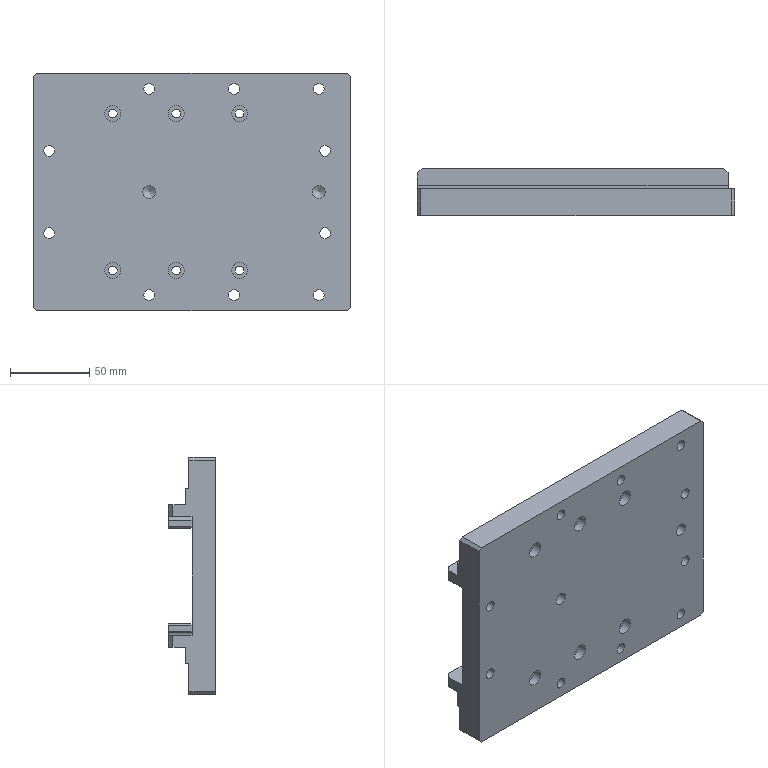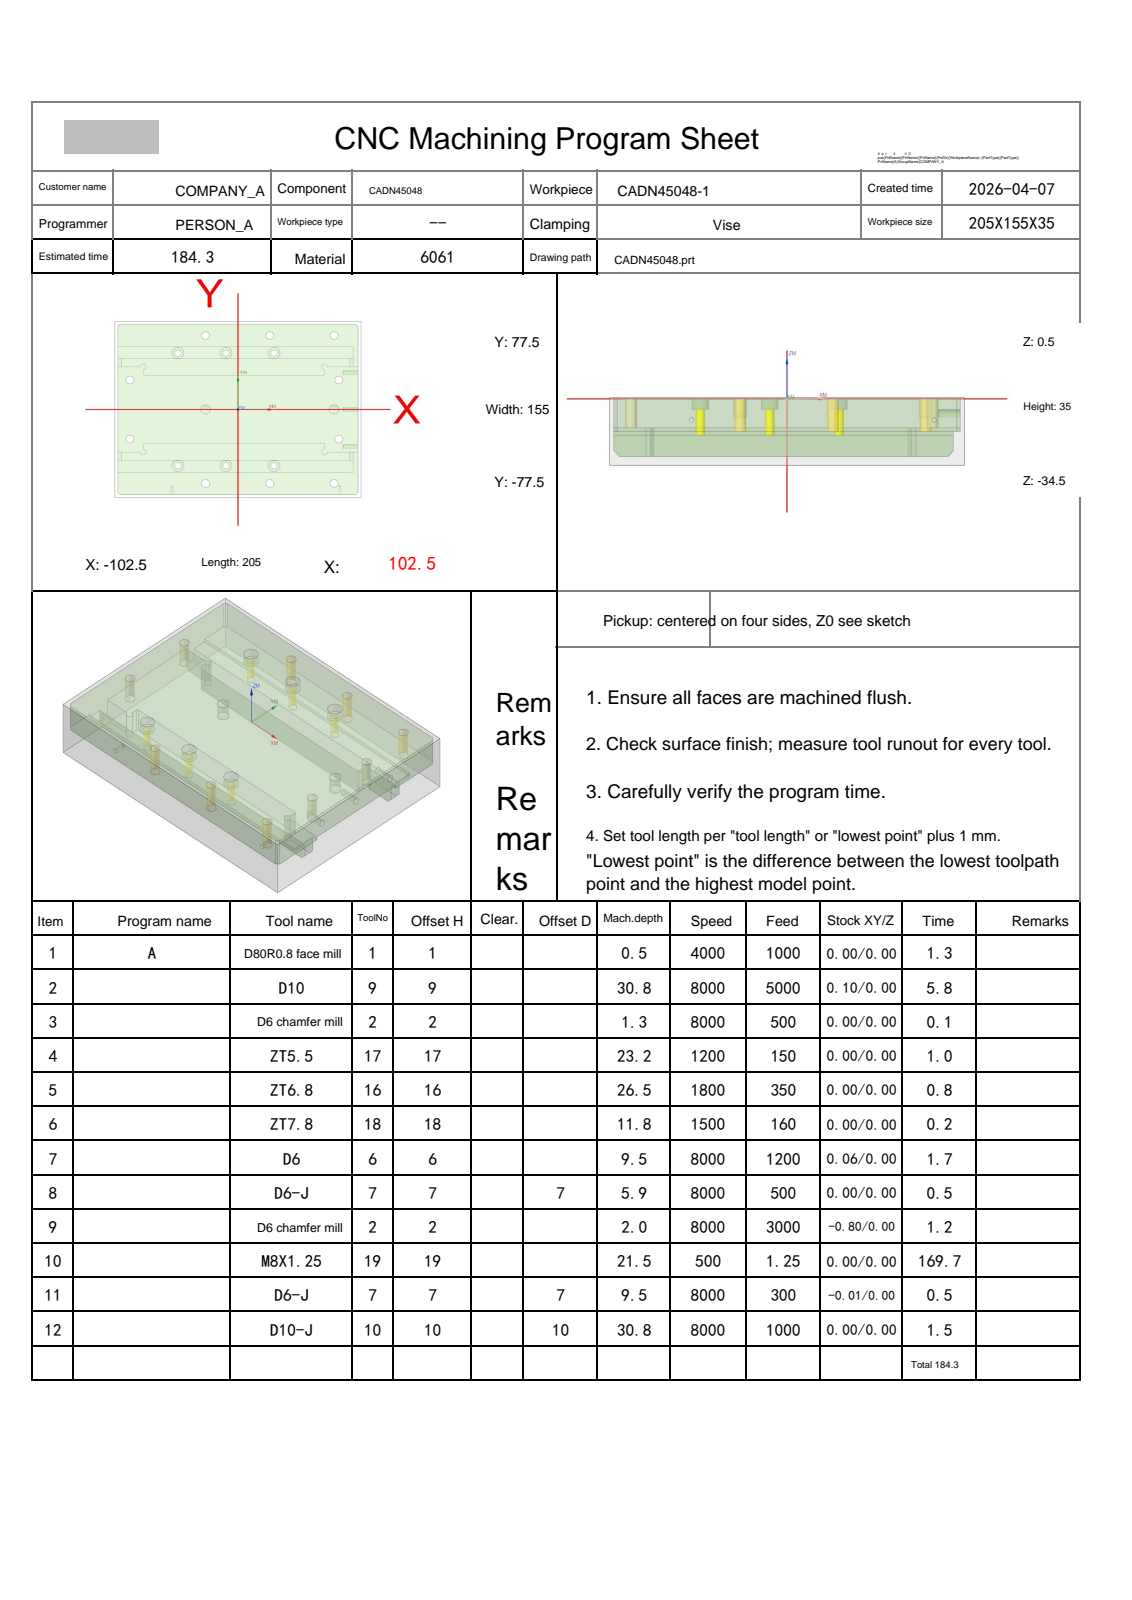NC program | NX | posted by the shop | part box 200 x 30 x 150 mm
Whole program, first 1289 of 1752 lines:
%
O0001
(Machine time: 348.05 MIN)
(===Total Tool:10===)
(T1=D80R0.8 face mill D=80.  R=0.8  D-  H01 Z=0.    )
(T9=D10     D=10.  R=0.   D-  H09 Z=-30.3 )
(T2=D6 chamfer mill   D=6.   R=0.   D-  H02 Z=-1.5  )
(T17=ZT5.5  D=5.5  DR_a=118 D-  H17 Z=-22.65)
(T16=ZT6.8  D=6.8  DR_a=118 D-  H16 Z=-26.04)
(T18=ZT7.8  D=7.8  DR_a=118 D-  H18 Z=-11.3 )
(T6=D6      D=6.   R=0.   D-  H06 Z=-9.   )
(T7=D6-J    D=6.   R=0.   D7  H07 Z=-9.   )
(T19=M8X1.25 D=6.8  DR_a=180 D-  H19 Z=-21.  )
(T10=D10-J  D=10.  R=0.   D10 H10 Z=-30.3 )
G80 G90 G17 G49 G40
G91 G28 Z0
M01
N1 T01 M06
(D80R0.8 face mill  D=80. R=0.8 H=01 ce=0.00 di=0.00)
G00 G90 G54 X145. Y-69. M03 S4000
G43 H01 Z20.
M08
Z2.
G01 Z0.0 F1000.
X140.
X-140.
Y-23.
X140.
Y23.
X-140.
Y69.
X140.
X145.
Z2.
G00 Z20.
G91 G28 Z0.0
M05
M09
G91 G28 Z0.0
M01
N2 T09 M06
(D10  D=10. R=0. H=09 ce=0.10 di=0.00)
G00 G90 G54 X0.0 Y-80.1 M03 S8000
G43 H09 Z20.
M08
Z.5
G01 X-98. Z.394 F5000.
G02 X-101.606 Y-78.606 Z.389 I0.0 J5.1
G01 X-103.606 Y-76.606 Z.386
G02 X-104.879 Y-74.486 Z.383 I3.606 J3.606
X-105.1 Y-73. Z.382 I4.879 J1.486
G01 Y73. Z.223
G02 X-103.606 Y76.606 Z.219 I5.1 J0.0
G01 X-101.606 Y78.606 Z.216
G02 X-98. Y80.1 Z.212 I3.606 J-3.606
G01 X98. Z-.001
G02 X101.606 Y78.606 Z-.006 I0.0 J-5.1
G01 X103.606 Y76.606 Z-.009
G02 X105.1 Y73. Z-.013 I-3.606 J-3.606
G01 Y-73. Z-.172
G02 X103.606 Y-76.606 Z-.176 I-5.1 J0.0
G01 X101.606 Y-78.606 Z-.179
G02 X98. Y-80.1 Z-.183 I-3.606 J3.606
G01 X-98. Z-.396
G02 X-101.606 Y-78.606 Z-.4 I0.0 J5.1
G01 X-103.606 Y-76.606 Z-.404
G02 X-104.879 Y-74.486 Z-.406 I3.606 J3.606
X-105.1 Y-73. Z-.408 I4.879 J1.486
G01 Y73. Z-.566
G02 X-103.606 Y76.606 Z-.571 I5.1 J0.0
G01 X-101.606 Y78.606 Z-.574
G02 X-98. Y80.1 Z-.578 I3.606 J-3.606
G01 X98. Z-.791
G02 X101.606 Y78.606 Z-.795 I0.0 J-5.1
G01 X103.606 Y76.606 Z-.798
G02 X105.1 Y73. Z-.803 I-3.606 J-3.606
G01 Y-73. Z-.961
G02 X103.606 Y-76.606 Z-.966 I-5.1 J0.0
G01 X101.606 Y-78.606 Z-.969
G02 X98. Y-80.1 Z-.973 I-3.606 J3.606
G01 X-98. Z-1.186
G02 X-101.606 Y-78.606 Z-1.19 I0.0 J5.1
G01 X-103.606 Y-76.606 Z-1.193
G02 X-104.879 Y-74.486 Z-1.196 I3.606 J3.606
X-105.1 Y-73. Z-1.198 I4.879 J1.486
G01 Y73. Z-1.356
G02 X-103.606 Y76.606 Z-1.361 I5.1 J0.0
G01 X-101.606 Y78.606 Z-1.364
G02 X-98. Y80.1 Z-1.368 I3.606 J-3.606
G01 X98. Z-1.581
G02 X101.606 Y78.606 Z-1.585 I0.0 J-5.1
G01 X103.606 Y76.606 Z-1.588
G02 X105.1 Y73. Z-1.593 I-3.606 J-3.606
G01 Y-73. Z-1.751
G02 X103.606 Y-76.606 Z-1.755 I-5.1 J0.0
G01 X101.606 Y-78.606 Z-1.758
G02 X98. Y-80.1 Z-1.763 I-3.606 J3.606
G01 X-98. Z-1.976
G02 X-101.606 Y-78.606 Z-1.98 I0.0 J5.1
G01 X-103.606 Y-76.606 Z-1.983
G02 X-104.879 Y-74.486 Z-1.986 I3.606 J3.606
X-105.1 Y-73. Z-1.987 I4.879 J1.486
G01 Y73. Z-2.146
G02 X-103.606 Y76.606 Z-2.15 I5.1 J0.0
G01 X-101.606 Y78.606 Z-2.153
G02 X-98. Y80.1 Z-2.158 I3.606 J-3.606
G01 X98. Z-2.371
G02 X101.606 Y78.606 Z-2.375 I0.0 J-5.1
G01 X103.606 Y76.606 Z-2.378
G02 X105.1 Y73. Z-2.382 I-3.606 J-3.606
G01 Y-73. Z-2.541
G02 X103.606 Y-76.606 Z-2.545 I-5.1 J0.0
G01 X101.606 Y-78.606 Z-2.548
G02 X98. Y-80.1 Z-2.553 I-3.606 J3.606
G01 X-98. Z-2.765
G02 X-101.606 Y-78.606 Z-2.77 I0.0 J5.1
G01 X-103.606 Y-76.606 Z-2.773
G02 X-104.879 Y-74.486 Z-2.776 I3.606 J3.606
X-105.1 Y-73. Z-2.777 I4.879 J1.486
G01 Y73. Z-2.936
G02 X-103.606 Y76.606 Z-2.94 I5.1 J0.0
G01 X-101.606 Y78.606 Z-2.943
G02 X-98. Y80.1 Z-2.947 I3.606 J-3.606
G01 X98. Z-3.16
G02 X101.606 Y78.606 Z-3.165 I0.0 J-5.1
G01 X103.606 Y76.606 Z-3.168
G02 X105.1 Y73. Z-3.172 I-3.606 J-3.606
G01 Y-73. Z-3.331
G02 X103.606 Y-76.606 Z-3.335 I-5.1 J0.0
G01 X101.606 Y-78.606 Z-3.338
G02 X98. Y-80.1 Z-3.342 I-3.606 J3.606
G01 X-98. Z-3.555
G02 X-101.606 Y-78.606 Z-3.559 I0.0 J5.1
G01 X-103.606 Y-76.606 Z-3.563
G02 X-104.879 Y-74.486 Z-3.565 I3.606 J3.606
X-105.1 Y-73. Z-3.567 I4.879 J1.486
G01 Y73. Z-3.725
G02 X-103.606 Y76.606 Z-3.73 I5.1 J0.0
G01 X-101.606 Y78.606 Z-3.733
G02 X-98. Y80.1 Z-3.737 I3.606 J-3.606
G01 X98. Z-3.95
G02 X101.606 Y78.606 Z-3.954 I0.0 J-5.1
G01 X103.606 Y76.606 Z-3.957
G02 X105.1 Y73. Z-3.962 I-3.606 J-3.606
G01 Y-73. Z-4.12
G02 X103.606 Y-76.606 Z-4.125 I-5.1 J0.0
G01 X101.606 Y-78.606 Z-4.128
G02 X98. Y-80.1 Z-4.132 I-3.606 J3.606
G01 X-98. Z-4.345
G02 X-101.606 Y-78.606 Z-4.349 I0.0 J5.1
G01 X-103.606 Y-76.606 Z-4.352
G02 X-104.879 Y-74.486 Z-4.355 I3.606 J3.606
X-105.1 Y-73. Z-4.357 I4.879 J1.486
G01 Y73. Z-4.515
G02 X-103.606 Y76.606 Z-4.52 I5.1 J0.0
G01 X-101.606 Y78.606 Z-4.523
G02 X-98. Y80.1 Z-4.527 I3.606 J-3.606
G01 X98. Z-4.74
G02 X101.606 Y78.606 Z-4.744 I0.0 J-5.1
G01 X103.606 Y76.606 Z-4.747
G02 X105.1 Y73. Z-4.752 I-3.606 J-3.606
G01 Y-73. Z-4.91
G02 X103.606 Y-76.606 Z-4.914 I-5.1 J0.0
G01 X101.606 Y-78.606 Z-4.917
G02 X98. Y-80.1 Z-4.922 I-3.606 J3.606
G01 X-98. Z-5.135
G02 X-101.606 Y-78.606 Z-5.139 I0.0 J5.1
G01 X-103.606 Y-76.606 Z-5.142
G02 X-104.879 Y-74.486 Z-5.145 I3.606 J3.606
X-105.1 Y-73. Z-5.146 I4.879 J1.486
G01 Y73. Z-5.305
G02 X-103.606 Y76.606 Z-5.309 I5.1 J0.0
G01 X-101.606 Y78.606 Z-5.312
G02 X-98. Y80.1 Z-5.317 I3.606 J-3.606
G01 X98. Z-5.529
G02 X101.606 Y78.606 Z-5.534 I0.0 J-5.1
G01 X103.606 Y76.606 Z-5.537
G02 X105.1 Y73. Z-5.541 I-3.606 J-3.606
G01 Y-73. Z-5.7
G02 X103.606 Y-76.606 Z-5.704 I-5.1 J0.0
G01 X101.606 Y-78.606 Z-5.707
G02 X98. Y-80.1 Z-5.712 I-3.606 J3.606
G01 X-98. Z-5.924
G02 X-101.606 Y-78.606 Z-5.929 I0.0 J5.1
G01 X-103.606 Y-76.606 Z-5.932
G02 X-104.879 Y-74.486 Z-5.934 I3.606 J3.606
X-105.1 Y-73. Z-5.936 I4.879 J1.486
G01 Y73. Z-6.095
G02 X-103.606 Y76.606 Z-6.099 I5.1 J0.0
G01 X-101.606 Y78.606 Z-6.102
G02 X-98. Y80.1 Z-6.106 I3.606 J-3.606
G01 X98. Z-6.319
G02 X101.606 Y78.606 Z-6.324 I0.0 J-5.1
G01 X103.606 Y76.606 Z-6.327
G02 X105.1 Y73. Z-6.331 I-3.606 J-3.606
G01 Y-73. Z-6.49
G02 X103.606 Y-76.606 Z-6.494 I-5.1 J0.0
G01 X101.606 Y-78.606 Z-6.497
G02 X98. Y-80.1 Z-6.501 I-3.606 J3.606
G01 X-98. Z-6.714
G02 X-101.606 Y-78.606 Z-6.718 I0.0 J5.1
G01 X-103.606 Y-76.606 Z-6.722
G02 X-104.879 Y-74.486 Z-6.724 I3.606 J3.606
X-105.1 Y-73. Z-6.726 I4.879 J1.486
G01 Y73. Z-6.884
G02 X-103.606 Y76.606 Z-6.889 I5.1 J0.0
G01 X-101.606 Y78.606 Z-6.892
G02 X-98. Y80.1 Z-6.896 I3.606 J-3.606
G01 X98. Z-7.109
G02 X101.606 Y78.606 Z-7.113 I0.0 J-5.1
G01 X103.606 Y76.606 Z-7.116
G02 X105.1 Y73. Z-7.121 I-3.606 J-3.606
G01 Y-73. Z-7.279
G02 X103.606 Y-76.606 Z-7.284 I-5.1 J0.0
G01 X101.606 Y-78.606 Z-7.287
G02 X98. Y-80.1 Z-7.291 I-3.606 J3.606
G01 X-98. Z-7.504
G02 X-101.606 Y-78.606 Z-7.508 I0.0 J5.1
G01 X-103.606 Y-76.606 Z-7.511
G02 X-104.879 Y-74.486 Z-7.514 I3.606 J3.606
X-105.1 Y-73. Z-7.516 I4.879 J1.486
G01 Y73. Z-7.674
G02 X-103.606 Y76.606 Z-7.678 I5.1 J0.0
G01 X-101.606 Y78.606 Z-7.682
G02 X-98. Y80.1 Z-7.686 I3.606 J-3.606
G01 X98. Z-7.899
G02 X101.606 Y78.606 Z-7.903 I0.0 J-5.1
G01 X103.606 Y76.606 Z-7.906
G02 X105.1 Y73. Z-7.91 I-3.606 J-3.606
G01 Y-73. Z-8.069
G02 X103.606 Y-76.606 Z-8.073 I-5.1 J0.0
G01 X101.606 Y-78.606 Z-8.076
G02 X98. Y-80.1 Z-8.081 I-3.606 J3.606
G01 X-98. Z-8.294
G02 X-101.606 Y-78.606 Z-8.298 I0.0 J5.1
G01 X-103.606 Y-76.606 Z-8.301
G02 X-104.879 Y-74.486 Z-8.304 I3.606 J3.606
X-105.1 Y-73. Z-8.305 I4.879 J1.486
G01 Y73. Z-8.464
G02 X-103.606 Y76.606 Z-8.468 I5.1 J0.0
G01 X-101.606 Y78.606 Z-8.471
G02 X-98. Y80.1 Z-8.476 I3.606 J-3.606
G01 X98. Z-8.688
G02 X101.606 Y78.606 Z-8.693 I0.0 J-5.1
G01 X103.606 Y76.606 Z-8.696
G02 X105.1 Y73. Z-8.7 I-3.606 J-3.606
G01 Y-73. Z-8.859
G02 X103.606 Y-76.606 Z-8.863 I-5.1 J0.0
G01 X101.606 Y-78.606 Z-8.866
G02 X98. Y-80.1 Z-8.871 I-3.606 J3.606
G01 X-98. Z-9.083
G02 X-101.606 Y-78.606 Z-9.088 I0.0 J5.1
G01 X-103.606 Y-76.606 Z-9.091
G02 X-104.879 Y-74.486 Z-9.093 I3.606 J3.606
X-105.1 Y-73. Z-9.095 I4.879 J1.486
G01 Y73. Z-9.254
G02 X-103.606 Y76.606 Z-9.258 I5.1 J0.0
G01 X-101.606 Y78.606 Z-9.261
G02 X-98. Y80.1 Z-9.265 I3.606 J-3.606
G01 X98. Z-9.478
G02 X101.606 Y78.606 Z-9.483 I0.0 J-5.1
G01 X103.606 Y76.606 Z-9.486
G02 X105.1 Y73. Z-9.49 I-3.606 J-3.606
G01 Y-73. Z-9.648
G02 X103.606 Y-76.606 Z-9.653 I-5.1 J0.0
G01 X101.606 Y-78.606 Z-9.656
G02 X98. Y-80.1 Z-9.66 I-3.606 J3.606
G01 X-98. Z-9.873
G02 X-101.606 Y-78.606 Z-9.877 I0.0 J5.1
G01 X-103.606 Y-76.606 Z-9.88
G02 X-104.879 Y-74.486 Z-9.883 I3.606 J3.606
X-105.1 Y-73. Z-9.885 I4.879 J1.486
G01 Y73. Z-10.043
G02 X-103.606 Y76.606 Z-10.048 I5.1 J0.0
G01 X-101.606 Y78.606 Z-10.051
G02 X-98. Y80.1 Z-10.055 I3.606 J-3.606
G01 X98. Z-10.268
G02 X101.606 Y78.606 Z-10.272 I0.0 J-5.1
G01 X103.606 Y76.606 Z-10.275
G02 X105.1 Y73. Z-10.28 I-3.606 J-3.606
G01 Y-73. Z-10.438
G02 X103.606 Y-76.606 Z-10.443 I-5.1 J0.0
G01 X101.606 Y-78.606 Z-10.446
G02 X98. Y-80.1 Z-10.45 I-3.606 J3.606
G01 X-98. Z-10.663
G02 X-101.606 Y-78.606 Z-10.667 I0.0 J5.1
G01 X-103.606 Y-76.606 Z-10.67
G02 X-104.879 Y-74.486 Z-10.673 I3.606 J3.606
X-105.1 Y-73. Z-10.675 I4.879 J1.486
G01 Y73. Z-10.833
G02 X-103.606 Y76.606 Z-10.837 I5.1 J0.0
G01 X-101.606 Y78.606 Z-10.841
G02 X-98. Y80.1 Z-10.845 I3.606 J-3.606
G01 X98. Z-11.058
G02 X101.606 Y78.606 Z-11.062 I0.0 J-5.1
G01 X103.606 Y76.606 Z-11.065
G02 X105.1 Y73. Z-11.069 I-3.606 J-3.606
G01 Y-73. Z-11.228
G02 X103.606 Y-76.606 Z-11.232 I-5.1 J0.0
G01 X101.606 Y-78.606 Z-11.235
G02 X98. Y-80.1 Z-11.24 I-3.606 J3.606
G01 X-98. Z-11.453
G02 X-101.606 Y-78.606 Z-11.457 I0.0 J5.1
G01 X-103.606 Y-76.606 Z-11.46
G02 X-104.879 Y-74.486 Z-11.463 I3.606 J3.606
X-105.1 Y-73. Z-11.464 I4.879 J1.486
G01 Y73. Z-11.623
G02 X-103.606 Y76.606 Z-11.627 I5.1 J0.0
G01 X-101.606 Y78.606 Z-11.63
G02 X-98. Y80.1 Z-11.635 I3.606 J-3.606
G01 X98. Z-11.847
G02 X101.606 Y78.606 Z-11.852 I0.0 J-5.1
G01 X103.606 Y76.606 Z-11.855
G02 X105.1 Y73. Z-11.859 I-3.606 J-3.606
G01 Y-73. Z-12.018
G02 X103.606 Y-76.606 Z-12.022 I-5.1 J0.0
G01 X101.606 Y-78.606 Z-12.025
G02 X98. Y-80.1 Z-12.029 I-3.606 J3.606
G01 X-98. Z-12.242
G02 X-101.606 Y-78.606 Z-12.247 I0.0 J5.1
G01 X-103.606 Y-76.606 Z-12.25
G02 X-104.879 Y-74.486 Z-12.252 I3.606 J3.606
X-105.1 Y-73. Z-12.254 I4.879 J1.486
G01 Y73. Z-12.413
G02 X-103.606 Y76.606 Z-12.417 I5.1 J0.0
G01 X-101.606 Y78.606 Z-12.42
G02 X-98. Y80.1 Z-12.424 I3.606 J-3.606
G01 X98. Z-12.637
G02 X101.606 Y78.606 Z-12.642 I0.0 J-5.1
G01 X103.606 Y76.606 Z-12.645
G02 X105.1 Y73. Z-12.649 I-3.606 J-3.606
G01 Y-73. Z-12.807
G02 X103.606 Y-76.606 Z-12.812 I-5.1 J0.0
G01 X101.606 Y-78.606 Z-12.815
G02 X98. Y-80.1 Z-12.819 I-3.606 J3.606
G01 X-98. Z-13.032
G02 X-101.606 Y-78.606 Z-13.036 I0.0 J5.1
G01 X-103.606 Y-76.606 Z-13.039
G02 X-104.879 Y-74.486 Z-13.042 I3.606 J3.606
X-105.1 Y-73. Z-13.044 I4.879 J1.486
G01 Y73. Z-13.202
G02 X-103.606 Y76.606 Z-13.207 I5.1 J0.0
G01 X-101.606 Y78.606 Z-13.21
G02 X-98. Y80.1 Z-13.214 I3.606 J-3.606
G01 X98. Z-13.427
G02 X101.606 Y78.606 Z-13.431 I0.0 J-5.1
G01 X103.606 Y76.606 Z-13.434
G02 X105.1 Y73. Z-13.439 I-3.606 J-3.606
G01 Y-73. Z-13.597
G02 X103.606 Y-76.606 Z-13.602 I-5.1 J0.0
G01 X101.606 Y-78.606 Z-13.605
G02 X98. Y-80.1 Z-13.609 I-3.606 J3.606
G01 X-98. Z-13.822
G02 X-101.606 Y-78.606 Z-13.826 I0.0 J5.1
G01 X-103.606 Y-76.606 Z-13.829
G02 X-104.879 Y-74.486 Z-13.832 I3.606 J3.606
X-105.1 Y-73. Z-13.834 I4.879 J1.486
G01 Y73. Z-13.992
G02 X-103.606 Y76.606 Z-13.996 I5.1 J0.0
G01 X-101.606 Y78.606 Z-14.
G02 X-98. Y80.1 Z-14.004 I3.606 J-3.606
G01 X98. Z-14.217
G02 X101.606 Y78.606 Z-14.221 I0.0 J-5.1
G01 X103.606 Y76.606 Z-14.224
G02 X105.1 Y73. Z-14.228 I-3.606 J-3.606
G01 Y-73. Z-14.387
G02 X103.606 Y-76.606 Z-14.391 I-5.1 J0.0
G01 X101.606 Y-78.606 Z-14.394
G02 X98. Y-80.1 Z-14.399 I-3.606 J3.606
G01 X-98. Z-14.612
G02 X-101.606 Y-78.606 Z-14.616 I0.0 J5.1
G01 X-103.606 Y-76.606 Z-14.619
G02 X-104.879 Y-74.486 Z-14.622 I3.606 J3.606
X-105.1 Y-73. Z-14.623 I4.879 J1.486
G01 Y73. Z-14.782
G02 X-103.606 Y76.606 Z-14.786 I5.1 J0.0
G01 X-101.606 Y78.606 Z-14.789
G02 X-98. Y80.1 Z-14.794 I3.606 J-3.606
G01 X98. Z-15.006
G02 X101.606 Y78.606 Z-15.011 I0.0 J-5.1
G01 X103.606 Y76.606 Z-15.014
G02 X105.1 Y73. Z-15.018 I-3.606 J-3.606
G01 Y-73. Z-15.177
G02 X103.606 Y-76.606 Z-15.181 I-5.1 J0.0
G01 X101.606 Y-78.606 Z-15.184
G02 X98. Y-80.1 Z-15.188 I-3.606 J3.606
G01 X-98. Z-15.401
G02 X-101.606 Y-78.606 Z-15.406 I0.0 J5.1
G01 X-103.606 Y-76.606 Z-15.409
G02 X-104.879 Y-74.486 Z-15.411 I3.606 J3.606
X-105.1 Y-73. Z-15.413 I4.879 J1.486
G01 Y73. Z-15.572
G02 X-103.606 Y76.606 Z-15.576 I5.1 J0.0
G01 X-101.606 Y78.606 Z-15.579
G02 X-98. Y80.1 Z-15.583 I3.606 J-3.606
G01 X98. Z-15.796
G02 X101.606 Y78.606 Z-15.8 I0.0 J-5.1
G01 X103.606 Y76.606 Z-15.804
G02 X105.1 Y73. Z-15.808 I-3.606 J-3.606
G01 Y-73. Z-15.966
G02 X103.606 Y-76.606 Z-15.971 I-5.1 J0.0
G01 X101.606 Y-78.606 Z-15.974
G02 X98. Y-80.1 Z-15.978 I-3.606 J3.606
G01 X-98. Z-16.191
G02 X-101.606 Y-78.606 Z-16.195 I0.0 J5.1
G01 X-103.606 Y-76.606 Z-16.198
G02 X-104.879 Y-74.486 Z-16.201 I3.606 J3.606
X-105.1 Y-73. Z-16.203 I4.879 J1.486
G01 Y73. Z-16.361
G02 X-103.606 Y76.606 Z-16.366 I5.1 J0.0
G01 X-101.606 Y78.606 Z-16.369
G02 X-98. Y80.1 Z-16.373 I3.606 J-3.606
G01 X98. Z-16.586
G02 X101.606 Y78.606 Z-16.59 I0.0 J-5.1
G01 X103.606 Y76.606 Z-16.593
G02 X105.1 Y73. Z-16.598 I-3.606 J-3.606
G01 Y-73. Z-16.756
G02 X103.606 Y-76.606 Z-16.761 I-5.1 J0.0
G01 X101.606 Y-78.606 Z-16.764
G02 X98. Y-80.1 Z-16.768 I-3.606 J3.606
G01 X-98. Z-16.981
G02 X-101.606 Y-78.606 Z-16.985 I0.0 J5.1
G01 X-103.606 Y-76.606 Z-16.988
G02 X-104.879 Y-74.486 Z-16.991 I3.606 J3.606
X-105.1 Y-73. Z-16.993 I4.879 J1.486
G01 Y73. Z-17.151
G02 X-103.606 Y76.606 Z-17.155 I5.1 J0.0
G01 X-101.606 Y78.606 Z-17.158
G02 X-98. Y80.1 Z-17.163 I3.606 J-3.606
G01 X98. Z-17.376
G02 X101.606 Y78.606 Z-17.38 I0.0 J-5.1
G01 X103.606 Y76.606 Z-17.383
G02 X105.1 Y73. Z-17.387 I-3.606 J-3.606
G01 Y-73. Z-17.546
G02 X103.606 Y-76.606 Z-17.55 I-5.1 J0.0
G01 X101.606 Y-78.606 Z-17.553
G02 X98. Y-80.1 Z-17.558 I-3.606 J3.606
G01 X-98. Z-17.771
G02 X-101.606 Y-78.606 Z-17.775 I0.0 J5.1
G01 X-103.606 Y-76.606 Z-17.778
G02 X-104.879 Y-74.486 Z-17.781 I3.606 J3.606
X-105.1 Y-73. Z-17.782 I4.879 J1.486
G01 Y73. Z-17.941
G02 X-103.606 Y76.606 Z-17.945 I5.1 J0.0
G01 X-101.606 Y78.606 Z-17.948
G02 X-98. Y80.1 Z-17.953 I3.606 J-3.606
G01 X98. Z-18.165
G02 X101.606 Y78.606 Z-18.17 I0.0 J-5.1
G01 X103.606 Y76.606 Z-18.173
G02 X105.1 Y73. Z-18.177 I-3.606 J-3.606
G01 Y-73. Z-18.336
G02 X103.606 Y-76.606 Z-18.34 I-5.1 J0.0
G01 X101.606 Y-78.606 Z-18.343
G02 X98. Y-80.1 Z-18.347 I-3.606 J3.606
G01 X-98. Z-18.56
G02 X-101.606 Y-78.606 Z-18.565 I0.0 J5.1
G01 X-103.606 Y-76.606 Z-18.568
G02 X-104.879 Y-74.486 Z-18.57 I3.606 J3.606
X-105.1 Y-73. Z-18.572 I4.879 J1.486
G01 Y73. Z-18.731
G02 X-103.606 Y76.606 Z-18.735 I5.1 J0.0
G01 X-101.606 Y78.606 Z-18.738
G02 X-98. Y80.1 Z-18.742 I3.606 J-3.606
G01 X98. Z-18.955
G02 X101.606 Y78.606 Z-18.959 I0.0 J-5.1
G01 X103.606 Y76.606 Z-18.963
G02 X105.1 Y73. Z-18.967 I-3.606 J-3.606
G01 Y-73. Z-19.125
G02 X103.606 Y-76.606 Z-19.13 I-5.1 J0.0
G01 X101.606 Y-78.606 Z-19.133
G02 X98. Y-80.1 Z-19.137 I-3.606 J3.606
G01 X-98. Z-19.35
G02 X-101.606 Y-78.606 Z-19.354 I0.0 J5.1
G01 X-103.606 Y-76.606 Z-19.357
G02 X-104.879 Y-74.486 Z-19.36 I3.606 J3.606
X-105.1 Y-73. Z-19.362 I4.879 J1.486
G01 Y73. Z-19.52
G02 X-103.606 Y76.606 Z-19.525 I5.1 J0.0
G01 X-101.606 Y78.606 Z-19.528
G02 X-98. Y80.1 Z-19.532 I3.606 J-3.606
G01 X98. Z-19.745
G02 X101.606 Y78.606 Z-19.749 I0.0 J-5.1
G01 X103.606 Y76.606 Z-19.752
G02 X105.1 Y73. Z-19.757 I-3.606 J-3.606
G01 Y-73. Z-19.915
G02 X103.606 Y-76.606 Z-19.92 I-5.1 J0.0
G01 X101.606 Y-78.606 Z-19.923
G02 X98. Y-80.1 Z-19.927 I-3.606 J3.606
G01 X-98. Z-20.14
G02 X-101.606 Y-78.606 Z-20.144 I0.0 J5.1
G01 X-103.606 Y-76.606 Z-20.147
G02 X-104.879 Y-74.486 Z-20.15 I3.606 J3.606
X-105.1 Y-73. Z-20.152 I4.879 J1.486
G01 Y73. Z-20.31
G02 X-103.606 Y76.606 Z-20.314 I5.1 J0.0
G01 X-101.606 Y78.606 Z-20.317
G02 X-98. Y80.1 Z-20.322 I3.606 J-3.606
G01 X98. Z-20.535
G02 X101.606 Y78.606 Z-20.539 I0.0 J-5.1
G01 X103.606 Y76.606 Z-20.542
G02 X105.1 Y73. Z-20.546 I-3.606 J-3.606
G01 Y-73. Z-20.705
G02 X103.606 Y-76.606 Z-20.709 I-5.1 J0.0
G01 X101.606 Y-78.606 Z-20.712
G02 X98. Y-80.1 Z-20.717 I-3.606 J3.606
G01 X-98. Z-20.929
G02 X-101.606 Y-78.606 Z-20.934 I0.0 J5.1
G01 X-103.606 Y-76.606 Z-20.937
G02 X-104.879 Y-74.486 Z-20.94 I3.606 J3.606
X-105.1 Y-73. Z-20.941 I4.879 J1.486
G01 Y73. Z-21.1
G02 X-103.606 Y76.606 Z-21.104 I5.1 J0.0
G01 X-101.606 Y78.606 Z-21.107
G02 X-98. Y80.1 Z-21.112 I3.606 J-3.606
G01 X98. Z-21.324
G02 X101.606 Y78.606 Z-21.329 I0.0 J-5.1
G01 X103.606 Y76.606 Z-21.332
G02 X105.1 Y73. Z-21.336 I-3.606 J-3.606
G01 Y-73. Z-21.495
G02 X103.606 Y-76.606 Z-21.499 I-5.1 J0.0
G01 X101.606 Y-78.606 Z-21.502
G02 X98. Y-80.1 Z-21.506 I-3.606 J3.606
G01 X-98. Z-21.719
G02 X-101.606 Y-78.606 Z-21.724 I0.0 J5.1
G01 X-103.606 Y-76.606 Z-21.727
G02 X-104.879 Y-74.486 Z-21.729 I3.606 J3.606
X-105.1 Y-73. Z-21.731 I4.879 J1.486
G01 Y73. Z-21.89
G02 X-103.606 Y76.606 Z-21.894 I5.1 J0.0
G01 X-101.606 Y78.606 Z-21.897
G02 X-98. Y80.1 Z-21.901 I3.606 J-3.606
G01 X98. Z-22.114
G02 X101.606 Y78.606 Z-22.118 I0.0 J-5.1
G01 X103.606 Y76.606 Z-22.122
G02 X105.1 Y73. Z-22.126 I-3.606 J-3.606
G01 Y-73. Z-22.284
G02 X103.606 Y-76.606 Z-22.289 I-5.1 J0.0
G01 X101.606 Y-78.606 Z-22.292
G02 X98. Y-80.1 Z-22.296 I-3.606 J3.606
G01 X-98. Z-22.509
G02 X-101.606 Y-78.606 Z-22.513 I0.0 J5.1
G01 X-103.606 Y-76.606 Z-22.516
G02 X-104.879 Y-74.486 Z-22.519 I3.606 J3.606
X-105.1 Y-73. Z-22.521 I4.879 J1.486
G01 Y73. Z-22.679
G02 X-103.606 Y76.606 Z-22.684 I5.1 J0.0
G01 X-101.606 Y78.606 Z-22.687
G02 X-98. Y80.1 Z-22.691 I3.606 J-3.606
G01 X98. Z-22.904
G02 X101.606 Y78.606 Z-22.908 I0.0 J-5.1
G01 X103.606 Y76.606 Z-22.911
G02 X105.1 Y73. Z-22.916 I-3.606 J-3.606
G01 Y-73. Z-23.074
G02 X103.606 Y-76.606 Z-23.078 I-5.1 J0.0
G01 X101.606 Y-78.606 Z-23.082
G02 X98. Y-80.1 Z-23.086 I-3.606 J3.606
G01 X-98. Z-23.299
G02 X-101.606 Y-78.606 Z-23.303 I0.0 J5.1
G01 X-103.606 Y-76.606 Z-23.306
G02 X-104.879 Y-74.486 Z-23.309 I3.606 J3.606
X-105.1 Y-73. Z-23.31 I4.879 J1.486
G01 Y73. Z-23.469
G02 X-103.606 Y76.606 Z-23.473 I5.1 J0.0
G01 X-101.606 Y78.606 Z-23.476
G02 X-98. Y80.1 Z-23.481 I3.606 J-3.606
G01 X98. Z-23.694
G02 X101.606 Y78.606 Z-23.698 I0.0 J-5.1
G01 X103.606 Y76.606 Z-23.701
G02 X105.1 Y73. Z-23.705 I-3.606 J-3.606
G01 Y-73. Z-23.864
G02 X103.606 Y-76.606 Z-23.868 I-5.1 J0.0
G01 X101.606 Y-78.606 Z-23.871
G02 X98. Y-80.1 Z-23.876 I-3.606 J3.606
G01 X-98. Z-24.088
G02 X-101.606 Y-78.606 Z-24.093 I0.0 J5.1
G01 X-103.606 Y-76.606 Z-24.096
G02 X-104.879 Y-74.486 Z-24.099 I3.606 J3.606
X-105.1 Y-73. Z-24.1 I4.879 J1.486
G01 Y73. Z-24.259
G02 X-103.606 Y76.606 Z-24.263 I5.1 J0.0
G01 X-101.606 Y78.606 Z-24.266
G02 X-98. Y80.1 Z-24.271 I3.606 J-3.606
G01 X98. Z-24.483
G02 X101.606 Y78.606 Z-24.488 I0.0 J-5.1
G01 X103.606 Y76.606 Z-24.491
G02 X105.1 Y73. Z-24.495 I-3.606 J-3.606
G01 Y-73. Z-24.654
G02 X103.606 Y-76.606 Z-24.658 I-5.1 J0.0
G01 X101.606 Y-78.606 Z-24.661
G02 X98. Y-80.1 Z-24.665 I-3.606 J3.606
G01 X-98. Z-24.878
G02 X-101.606 Y-78.606 Z-24.883 I0.0 J5.1
G01 X-103.606 Y-76.606 Z-24.886
G02 X-104.879 Y-74.486 Z-24.888 I3.606 J3.606
X-105.1 Y-73. Z-24.89 I4.879 J1.486
G01 Y73. Z-25.048
G02 X-103.606 Y76.606 Z-25.053 I5.1 J0.0
G01 X-101.606 Y78.606 Z-25.056
G02 X-98. Y80.1 Z-25.06 I3.606 J-3.606
G01 X98. Z-25.273
G02 X101.606 Y78.606 Z-25.277 I0.0 J-5.1
G01 X103.606 Y76.606 Z-25.28
G02 X105.1 Y73. Z-25.285 I-3.606 J-3.606
G01 Y-73. Z-25.443
G02 X103.606 Y-76.606 Z-25.448 I-5.1 J0.0
G01 X101.606 Y-78.606 Z-25.451
G02 X98. Y-80.1 Z-25.455 I-3.606 J3.606
G01 X-98. Z-25.668
G02 X-101.606 Y-78.606 Z-25.672 I0.0 J5.1
G01 X-103.606 Y-76.606 Z-25.675
G02 X-104.879 Y-74.486 Z-25.678 I3.606 J3.606
X-105.1 Y-73. Z-25.68 I4.879 J1.486
G01 Y73. Z-25.838
G02 X-103.606 Y76.606 Z-25.843 I5.1 J0.0
G01 X-101.606 Y78.606 Z-25.846
G02 X-98. Y80.1 Z-25.85 I3.606 J-3.606
G01 X98. Z-26.063
G02 X101.606 Y78.606 Z-26.067 I0.0 J-5.1
G01 X103.606 Y76.606 Z-26.07
G02 X105.1 Y73. Z-26.075 I-3.606 J-3.606
G01 Y-73. Z-26.233
G02 X103.606 Y-76.606 Z-26.237 I-5.1 J0.0
G01 X101.606 Y-78.606 Z-26.241
G02 X98. Y-80.1 Z-26.245 I-3.606 J3.606
G01 X-98. Z-26.458
G02 X-101.606 Y-78.606 Z-26.462 I0.0 J5.1
G01 X-103.606 Y-76.606 Z-26.465
G02 X-104.879 Y-74.486 Z-26.468 I3.606 J3.606
X-105.1 Y-73. Z-26.469 I4.879 J1.486
G01 Y73. Z-26.628
G02 X-103.606 Y76.606 Z-26.632 I5.1 J0.0
G01 X-101.606 Y78.606 Z-26.635
G02 X-98. Y80.1 Z-26.64 I3.606 J-3.606
G01 X98. Z-26.853
G02 X101.606 Y78.606 Z-26.857 I0.0 J-5.1
G01 X103.606 Y76.606 Z-26.86
G02 X105.1 Y73. Z-26.864 I-3.606 J-3.606
G01 Y-73. Z-27.023
G02 X103.606 Y-76.606 Z-27.027 I-5.1 J0.0
G01 X101.606 Y-78.606 Z-27.03
G02 X98. Y-80.1 Z-27.035 I-3.606 J3.606
G01 X-98. Z-27.247
G02 X-101.606 Y-78.606 Z-27.252 I0.0 J5.1
G01 X-103.606 Y-76.606 Z-27.255
G02 X-104.879 Y-74.486 Z-27.258 I3.606 J3.606
X-105.1 Y-73. Z-27.259 I4.879 J1.486
G01 Y73. Z-27.418
G02 X-103.606 Y76.606 Z-27.422 I5.1 J0.0
G01 X-101.606 Y78.606 Z-27.425
G02 X-98. Y80.1 Z-27.429 I3.606 J-3.606
G01 X98. Z-27.642
G02 X101.606 Y78.606 Z-27.647 I0.0 J-5.1
G01 X103.606 Y76.606 Z-27.65
G02 X105.1 Y73. Z-27.654 I-3.606 J-3.606
G01 Y-73. Z-27.813
G02 X103.606 Y-76.606 Z-27.817 I-5.1 J0.0
G01 X101.606 Y-78.606 Z-27.82
G02 X98. Y-80.1 Z-27.824 I-3.606 J3.606
G01 X-98. Z-28.037
G02 X-101.606 Y-78.606 Z-28.042 I0.0 J5.1
G01 X-103.606 Y-76.606 Z-28.045
G02 X-104.879 Y-74.486 Z-28.047 I3.606 J3.606
X-105.1 Y-73. Z-28.049 I4.879 J1.486
G01 Y73. Z-28.207
G02 X-103.606 Y76.606 Z-28.212 I5.1 J0.0
G01 X-101.606 Y78.606 Z-28.215
G02 X-98. Y80.1 Z-28.219 I3.606 J-3.606
G01 X98. Z-28.432
G02 X101.606 Y78.606 Z-28.436 I0.0 J-5.1
G01 X103.606 Y76.606 Z-28.439
G02 X105.1 Y73. Z-28.444 I-3.606 J-3.606
G01 Y-73. Z-28.602
G02 X103.606 Y-76.606 Z-28.607 I-5.1 J0.0
G01 X101.606 Y-78.606 Z-28.61
G02 X98. Y-80.1 Z-28.614 I-3.606 J3.606
G01 X-98. Z-28.827
G02 X-101.606 Y-78.606 Z-28.831 I0.0 J5.1
G01 X-103.606 Y-76.606 Z-28.834
G02 X-104.879 Y-74.486 Z-28.837 I3.606 J3.606
X-105.1 Y-73. Z-28.839 I4.879 J1.486
G01 Y73. Z-28.997
G02 X-103.606 Y76.606 Z-29.002 I5.1 J0.0
G01 X-101.606 Y78.606 Z-29.005
G02 X-98. Y80.1 Z-29.009 I3.606 J-3.606
G01 X98. Z-29.222
G02 X101.606 Y78.606 Z-29.226 I0.0 J-5.1
G01 X103.606 Y76.606 Z-29.229
G02 X105.1 Y73. Z-29.234 I-3.606 J-3.606
G01 Y-73. Z-29.392
G02 X103.606 Y-76.606 Z-29.396 I-5.1 J0.0
G01 X101.606 Y-78.606 Z-29.4
G02 X98. Y-80.1 Z-29.404 I-3.606 J3.606
G01 X-98. Z-29.617
G02 X-101.606 Y-78.606 Z-29.621 I0.0 J5.1
G01 X-103.606 Y-76.606 Z-29.624
G02 X-104.879 Y-74.486 Z-29.627 I3.606 J3.606
X-105.1 Y-73. Z-29.628 I4.879 J1.486
G01 Y73. Z-29.787
G02 X-103.606 Y76.606 Z-29.791 I5.1 J0.0
G01 X-101.606 Y78.606 Z-29.794
G02 X-98. Y80.1 Z-29.799 I3.606 J-3.606
G01 X98. Z-30.012
G02 X101.606 Y78.606 Z-30.016 I0.0 J-5.1
G01 X103.606 Y76.606 Z-30.019
G02 X105.1 Y73. Z-30.023 I-3.606 J-3.606
G01 Y-73. Z-30.182
G02 X103.606 Y-76.606 Z-30.186 I-5.1 J0.0
G01 X101.606 Y-78.606 Z-30.189
G02 X98. Y-80.1 Z-30.194 I-3.606 J3.606
G01 X0.0 Z-30.3
X-98.
G02 X-101.606 Y-78.606 I0.0 J5.1
G01 X-103.606 Y-76.606
G02 X-105.1 Y-73. I3.606 J3.606
G01 Y73.
G02 X-103.606 Y76.606 I5.1 J0.0
G01 X-101.606 Y78.606
G02 X-98. Y80.1 I3.606 J-3.606
G01 X98.
G02 X101.606 Y78.606 I0.0 J-5.1
G01 X103.606 Y76.606
G02 X105.1 Y73. I-3.606 J-3.606
G01 Y-73.
G02 X103.606 Y-76.606 I-5.1 J0.0
G01 X101.606 Y-78.606
G02 X98. Y-80.1 I-3.606 J3.606
G01 X0.0
X-.5
Z-29.3
G00 Z20.
G91 G28 Z0.0
M05
M09
G91 G28 Z0.0
M01
N3 T02 M06
(D6 chamfer mill  D=6. R=0. H=02 ce=0.00 di=0.00)
G00 G90 G54 X-27. Y0.0 M03 S8000
G43 H02 Z20.
M08
G98 G81 X-27. Y0.0 Z-.8 R1. F500.
X-50. Y49.5
X-27. Y65.
X-10. Y49.5
X26.5 Y65.
X30. Y49.5
X80. Y65.
X84. Y26.
X80. Y0.0
X84. Y-26.
X80. Y-65.
X30. Y-49.5
X26.5 Y-65.
X-10. Y-49.5
X-27. Y-65.
X-50. Y-49.5
X-90. Y-26.
Y26.
G80
G00 Z20.
G91 G28 Z0.0
M05
M09
G91 G28 Z0.0
M01
N4 T17 M06
(ZT5.5 D=5.5 DR_a=118 H=17)
G00 G90 G54 X-50. Y-49.5 M03 S1200
G43 H17 Z20.
M08
G98 G83 X-50. Y-49.5 Z-22.652 R1. F150. Q2.
X-10.
X30.
Y49.5
X-10.
X-50.
G80
G00 Z20.
G91 G28 Z0.0
M05
M09
G91 G28 Z0.0
M01
N5 T16 M06
(ZT6.8 D=6.8 DR_a=118 H=16)
G00 G90 G54 X-27. Y-65. M03 S1800
G43 H16 Z20.
M08
G98 G83 X-27. Y-65. Z-26.043 R1. F350. Q3.
X26.5
X80.
G98 G83 X84. Y-26. Z-24.043 R1. Q3.
Y26.
G98 G83 X80. Y65. Z-26.043 R1. Q3.
X26.5
X-27.
G98 G83 X-90. Y26. Z-24.043 R1. Q3.
Y-26.
G80
G00 Z20.
G91 G28 Z0.0
M05
M09
G91 G28 Z0.0
M01
N6 T18 M06
(ZT7.8 D=7.8 DR_a=118 H=18)
G00 G90 G54 X80. Y0.0 M03 S1500
G43 H18 Z20.
M08
G98 G83 X80. Y0.0 Z-11.303 R1. F160. Q2.
X-27.
G80
G00 Z20.
G91 G28 Z0.0
M05
M09
G91 G28 Z0.0
M01
N7 T06 M06
(D6  D=6. R=0. H=06 ce=0.06 di=0.00)
G00 G90 G54 X80. Y0.0 M03 S8000
G43 H06 Z20.
M08
Z.5
G03 X80.47 Y-.47 I.47 J0.0 F500.
X80.94 Y0.0 I0.0 J.47
X80.94 Y0.0 Z.2 I-.94 J0.0
X80.94 Y0.0 Z-.1 I-.94 J0.0
X80.94 Y0.0 Z-.4 I-.94 J0.0
X80.94 Y0.0 Z-.7 I-.94 J0.0
X80.94 Y0.0 Z-1. I-.94 J0.0
X80.94 Y0.0 Z-1.3 I-.94 J0.0
X80.94 Y0.0 Z-1.6 I-.94 J0.0
X80.94 Y0.0 Z-1.9 I-.94 J0.0
X80.94 Y0.0 Z-2.2 I-.94 J0.0
X80.94 Y0.0 Z-2.5 I-.94 J0.0
X80.94 Y0.0 Z-2.8 I-.94 J0.0
X80.94 Y0.0 Z-3.1 I-.94 J0.0
X80.94 Y0.0 Z-3.4 I-.94 J0.0
X80.94 Y0.0 Z-3.7 I-.94 J0.0
X80.94 Y0.0 Z-4. I-.94 J0.0
X80.94 Y0.0 Z-4.3 I-.94 J0.0
X80.94 Y0.0 Z-4.6 I-.94 J0.0
X80.94 Y0.0 Z-4.9 I-.94 J0.0
X80.94 Y0.0 Z-5.2 I-.94 J0.0
X80.94 Y0.0 Z-5.5 I-.94 J0.0
X80.94 Y0.0 Z-5.8 I-.94 J0.0
X80.94 Y0.0 Z-6.1 I-.94 J0.0
X80.94 Y0.0 Z-6.4 I-.94 J0.0
X80.94 Y0.0 Z-6.7 I-.94 J0.0
X80.94 Y0.0 Z-7. I-.94 J0.0
X80.94 Y0.0 Z-7.3 I-.94 J0.0
X80.94 Y0.0 Z-7.6 I-.94 J0.0
X80.94 Y0.0 Z-7.9 I-.94 J0.0
X80.94 Y0.0 Z-8.2 I-.94 J0.0
X80.94 Y0.0 Z-8.5 I-.94 J0.0
X80.94 Y0.0 Z-8.8 I-.94 J0.0
X79.53 Y-.814 Z-9. I-.94 J0.0
X80. Y-.94 I.47 J.814
X80.94 Y0.0 I0.0 J.94
X80. Y.94 I-.94 J0.0
X79.06 Y0.0 I0.0 J-.94
X79.53 Y-.814 I.94 J0.0
X79.765 Y-.877 I.235 J.407
X80.235 Y-.407 I0.0 J.47
X80. Y0.0 I-.47 J0.0
G00 Z20.
X-27.
Z.5
G03 X-26.53 Y-.47 I.47 J0.0
X-26.06 Y0.0 I0.0 J.47
X-26.06 Y0.0 Z.2 I-.94 J0.0
X-26.06 Y0.0 Z-.1 I-.94 J0.0
X-26.06 Y0.0 Z-.4 I-.94 J0.0
X-26.06 Y0.0 Z-.7 I-.94 J0.0
X-26.06 Y0.0 Z-1. I-.94 J0.0
X-26.06 Y0.0 Z-1.3 I-.94 J0.0
X-26.06 Y0.0 Z-1.6 I-.94 J0.0
X-26.06 Y0.0 Z-1.9 I-.94 J0.0
X-26.06 Y0.0 Z-2.2 I-.94 J0.0
X-26.06 Y0.0 Z-2.5 I-.94 J0.0
X-26.06 Y0.0 Z-2.8 I-.94 J0.0
X-26.06 Y0.0 Z-3.1 I-.94 J0.0
X-26.06 Y0.0 Z-3.4 I-.94 J0.0
X-26.06 Y0.0 Z-3.7 I-.94 J0.0
X-26.06 Y0.0 Z-4. I-.94 J0.0
X-26.06 Y0.0 Z-4.3 I-.94 J0.0
X-26.06 Y0.0 Z-4.6 I-.94 J0.0
X-26.06 Y0.0 Z-4.9 I-.94 J0.0
X-26.06 Y0.0 Z-5.2 I-.94 J0.0
X-26.06 Y0.0 Z-5.5 I-.94 J0.0
X-26.06 Y0.0 Z-5.8 I-.94 J0.0
X-26.06 Y0.0 Z-6.1 I-.94 J0.0
X-26.06 Y0.0 Z-6.4 I-.94 J0.0
X-26.06 Y0.0 Z-6.7 I-.94 J0.0
X-26.06 Y0.0 Z-7. I-.94 J0.0
X-26.06 Y0.0 Z-7.3 I-.94 J0.0
X-26.06 Y0.0 Z-7.6 I-.94 J0.0
X-26.06 Y0.0 Z-7.9 I-.94 J0.0
X-26.06 Y0.0 Z-8.2 I-.94 J0.0
X-26.06 Y0.0 Z-8.5 I-.94 J0.0
X-26.06 Y0.0 Z-8.8 I-.94 J0.0
X-27.47 Y-.814 Z-9. I-.94 J0.0
X-27. Y-.94 I.47 J.814
X-26.06 Y0.0 I0.0 J.94
X-27. Y.94 I-.94 J0.0
X-27.94 Y0.0 I0.0 J-.94
X-27.47 Y-.814 I.94 J0.0
X-27.235 Y-.877 I.235 J.407
X-26.765 Y-.407 I0.0 J.47
X-27. Y0.0 I-.47 J0.0
G00 Z20.
G00 G90 X-50. Y-49.5 M03 S8000
Z20.
Z.5
G03 X-49.05 Y-50.45 I.95 J0.0 F1200.
X-48.1 Y-49.5 I0.0 J.95
X-48.1 Y-49.5 Z0.0 I-1.9 J0.0
X-48.1 Y-49.5 Z-.5 I-1.9 J0.0
X-48.1 Y-49.5 Z-1. I-1.9 J0.0
X-48.1 Y-49.5 Z-1.5 I-1.9 J0.0
X-48.1 Y-49.5 Z-2. I-1.9 J0.0
X-48.1 Y-49.5 Z-2.5 I-1.9 J0.0
X-48.1 Y-49.5 Z-3. I-1.9 J0.0
X-48.1 Y-49.5 Z-3.5 I-1.9 J0.0
X-48.1 Y-49.5 Z-4. I-1.9 J0.0
X-48.1 Y-49.5 Z-4.5 I-1.9 J0.0
X-48.1 Y-49.5 Z-5. I-1.9 J0.0
X-49.413 Y-51.307 Z-5.4 I-1.9 J0.0
X-48.1 Y-49.5 I-.587 J1.807
X-50. Y-47.6 I-1.9 J0.0
X-51.9 Y-49.5 I0.0 J-1.9
X-50. Y-51.4 I1.9 J0.0
X-49.413 Y-51.307 I0.0 J1.9
X-48.756 Y-50.404 I-.294 J.904
X-49.706 Y-49.454 I-.95 J0.0
X-50. Y-49.5 I0.0 J-.95
G00 Z20.
X-10.
Z.5
G03 X-9.05 Y-50.45 I.95 J0.0
X-8.1 Y-49.5 I0.0 J.95
X-8.1 Y-49.5 Z0.0 I-1.9 J0.0
X-8.1 Y-49.5 Z-.5 I-1.9 J0.0
X-8.1 Y-49.5 Z-1. I-1.9 J0.0
X-8.1 Y-49.5 Z-1.5 I-1.9 J0.0
X-8.1 Y-49.5 Z-2. I-1.9 J0.0
X-8.1 Y-49.5 Z-2.5 I-1.9 J0.0
X-8.1 Y-49.5 Z-3. I-1.9 J0.0
X-8.1 Y-49.5 Z-3.5 I-1.9 J0.0
X-8.1 Y-49.5 Z-4. I-1.9 J0.0
X-8.1 Y-49.5 Z-4.5 I-1.9 J0.0
X-8.1 Y-49.5 Z-5. I-1.9 J0.0
X-9.413 Y-51.307 Z-5.4 I-1.9 J0.0
X-8.1 Y-49.5 I-.587 J1.807
X-10. Y-47.6 I-1.9 J0.0
X-11.9 Y-49.5 I0.0 J-1.9
X-10. Y-51.4 I1.9 J0.0
X-9.413 Y-51.307 I0.0 J1.9
X-8.756 Y-50.404 I-.294 J.904
X-9.706 Y-49.454 I-.95 J0.0
X-10. Y-49.5 I0.0 J-.95
G00 Z20.
X30.
Z.5
G03 X30.95 Y-50.45 I.95 J0.0
X31.9 Y-49.5 I0.0 J.95
X31.9 Y-49.5 Z0.0 I-1.9 J0.0
X31.9 Y-49.5 Z-.5 I-1.9 J0.0
X31.9 Y-49.5 Z-1. I-1.9 J0.0
X31.9 Y-49.5 Z-1.5 I-1.9 J0.0
X31.9 Y-49.5 Z-2. I-1.9 J0.0
X31.9 Y-49.5 Z-2.5 I-1.9 J0.0
X31.9 Y-49.5 Z-3. I-1.9 J0.0
X31.9 Y-49.5 Z-3.5 I-1.9 J0.0
X31.9 Y-49.5 Z-4. I-1.9 J0.0
X31.9 Y-49.5 Z-4.5 I-1.9 J0.0
X31.9 Y-49.5 Z-5. I-1.9 J0.0
X30.587 Y-51.307 Z-5.4 I-1.9 J0.0
X31.9 Y-49.5 I-.587 J1.807
X30. Y-47.6 I-1.9 J0.0
X28.1 Y-49.5 I0.0 J-1.9
X30. Y-51.4 I1.9 J0.0
X30.587 Y-51.307 I0.0 J1.9
X31.244 Y-50.404 I-.294 J.904
X30.294 Y-49.454 I-.95 J0.0
X30. Y-49.5 I0.0 J-.95
G00 Z20.
Y49.5
Z.5
G03 X30.95 Y48.55 I.95 J0.0
X31.9 Y49.5 I0.0 J.95
X31.9 Y49.5 Z0.0 I-1.9 J0.0
X31.9 Y49.5 Z-.5 I-1.9 J0.0
X31.9 Y49.5 Z-1. I-1.9 J0.0
X31.9 Y49.5 Z-1.5 I-1.9 J0.0
X31.9 Y49.5 Z-2. I-1.9 J0.0
X31.9 Y49.5 Z-2.5 I-1.9 J0.0
X31.9 Y49.5 Z-3. I-1.9 J0.0
X31.9 Y49.5 Z-3.5 I-1.9 J0.0
X31.9 Y49.5 Z-4. I-1.9 J0.0
X31.9 Y49.5 Z-4.5 I-1.9 J0.0
X31.9 Y49.5 Z-5. I-1.9 J0.0
X30.587 Y47.693 Z-5.4 I-1.9 J0.0
X31.9 Y49.5 I-.587 J1.807
X30. Y51.4 I-1.9 J0.0
X28.1 Y49.5 I0.0 J-1.9
X30. Y47.6 I1.9 J0.0
X30.587 Y47.693 I0.0 J1.9
X31.244 Y48.596 I-.294 J.904
X30.294 Y49.546 I-.95 J0.0
X30. Y49.5 I0.0 J-.95
G00 Z20.
X-10.
Z.5
G03 X-9.05 Y48.55 I.95 J0.0
X-8.1 Y49.5 I0.0 J.95
X-8.1 Y49.5 Z0.0 I-1.9 J0.0
X-8.1 Y49.5 Z-.5 I-1.9 J0.0
X-8.1 Y49.5 Z-1. I-1.9 J0.0
X-8.1 Y49.5 Z-1.5 I-1.9 J0.0
X-8.1 Y49.5 Z-2. I-1.9 J0.0
X-8.1 Y49.5 Z-2.5 I-1.9 J0.0
X-8.1 Y49.5 Z-3. I-1.9 J0.0
X-8.1 Y49.5 Z-3.5 I-1.9 J0.0
X-8.1 Y49.5 Z-4. I-1.9 J0.0
X-8.1 Y49.5 Z-4.5 I-1.9 J0.0
X-8.1 Y49.5 Z-5. I-1.9 J0.0
X-9.413 Y47.693 Z-5.4 I-1.9 J0.0
X-8.1 Y49.5 I-.587 J1.807
X-10. Y51.4 I-1.9 J0.0
X-11.9 Y49.5 I0.0 J-1.9
X-10. Y47.6 I1.9 J0.0
X-9.413 Y47.693 I0.0 J1.9
X-8.756 Y48.596 I-.294 J.904
X-9.706 Y49.546 I-.95 J0.0
X-10. Y49.5 I0.0 J-.95
G00 Z20.
X-50.
Z.5
G03 X-49.05 Y48.55 I.95 J0.0
X-48.1 Y49.5 I0.0 J.95
X-48.1 Y49.5 Z0.0 I-1.9 J0.0
X-48.1 Y49.5 Z-.5 I-1.9 J0.0
X-48.1 Y49.5 Z-1. I-1.9 J0.0
X-48.1 Y49.5 Z-1.5 I-1.9 J0.0
X-48.1 Y49.5 Z-2. I-1.9 J0.0
X-48.1 Y49.5 Z-2.5 I-1.9 J0.0
X-48.1 Y49.5 Z-3. I-1.9 J0.0
X-48.1 Y49.5 Z-3.5 I-1.9 J0.0
X-48.1 Y49.5 Z-4. I-1.9 J0.0
X-48.1 Y49.5 Z-4.5 I-1.9 J0.0
X-48.1 Y49.5 Z-5. I-1.9 J0.0
X-49.413 Y47.693 Z-5.4 I-1.9 J0.0
X-48.1 Y49.5 I-.587 J1.807
X-50. Y51.4 I-1.9 J0.0
X-51.9 Y49.5 I0.0 J-1.9
X-50. Y47.6 I1.9 J0.0
X-49.413 Y47.693 I0.0 J1.9
X-48.756 Y48.596 I-.294 J.904
X-49.706 Y49.546 I-.95 J0.0
X-50. Y49.5 I0.0 J-.95
G00 Z20.
G91 G28 Z0.0
M05
M09
G91 G28 Z0.0
M01
N8 T07 M06
(D6-J  D=6. R=0. H=07 ce=0.00 di=0.00)
G00 G90 G54 X-50. Y-49.5 M03 S8000
G43 H07 Z20.
M08
Z0.0
G41 D07
G01 X-49.96 Y-49.696 F500.
G03 X-48.99 Y-50.49 I.97 J.196
X-48. Y-49.5 I0.0 J.99
X-48. Y-49.5 Z-5. I-2. J0.0
X-48.247 Y-48.536 Z-5.4 I-2. J0.0
X-50. Y-47.5 I-1.753 J-.964
X-52. Y-49.5 I0.0 J-2.
X-50. Y-51.5 I2. J0.0
X-48. Y-49.5 I0.0 J2.
X-48.247 Y-48.536 I-2. J0.0
X-49.115 Y-48.023 I-.868 J-.477
X-50.105 Y-49.013 I0.0 J-.99
X-50.06 Y-49.309 I.99 J0.0
G01 G40 X-50. Y-49.5
G00 Z20.
X-10.
Z0.0
G41 D07
G01 X-9.96 Y-49.696
G03 X-8.99 Y-50.49 I.97 J.196
X-8. Y-49.5 I0.0 J.99
X-8. Y-49.5 Z-5. I-2. J0.0
X-8.247 Y-48.536 Z-5.4 I-2. J0.0
X-10. Y-47.5 I-1.753 J-.964
X-12. Y-49.5 I0.0 J-2.
X-10. Y-51.5 I2. J0.0
X-8. Y-49.5 I0.0 J2.
X-8.247 Y-48.536 I-2. J0.0
X-9.115 Y-48.023 I-.868 J-.477
X-10.105 Y-49.013 I0.0 J-.99
X-10.06 Y-49.309 I.99 J0.0
G01 G40 X-10. Y-49.5
G00 Z20.
X30.
Z0.0
G41 D07
G01 X30.04 Y-49.696
G03 X31.01 Y-50.49 I.97 J.196
X32. Y-49.5 I0.0 J.99
X32. Y-49.5 Z-5. I-2. J0.0
X31.753 Y-48.536 Z-5.4 I-2. J0.0
X30. Y-47.5 I-1.753 J-.964
X28. Y-49.5 I0.0 J-2.
X30. Y-51.5 I2. J0.0
X32. Y-49.5 I0.0 J2.
X31.753 Y-48.536 I-2. J0.0
X30.885 Y-48.023 I-.868 J-.477
X29.895 Y-49.013 I0.0 J-.99
X29.94 Y-49.309 I.99 J0.0
G01 G40 X30. Y-49.5
G00 Z20.
Y49.5
Z0.0
G41 D07
G01 X30.04 Y49.304
G03 X31.01 Y48.51 I.97 J.196
X32. Y49.5 I0.0 J.99
X32. Y49.5 Z-5. I-2. J0.0
X31.753 Y50.464 Z-5.4 I-2. J0.0
X30. Y51.5 I-1.753 J-.964
X28. Y49.5 I0.0 J-2.
X30. Y47.5 I2. J0.0
X32. Y49.5 I0.0 J2.
X31.753 Y50.464 I-2. J0.0
X30.885 Y50.977 I-.868 J-.477
X29.895 Y49.987 I0.0 J-.99
X29.94 Y49.691 I.99 J0.0
G01 G40 X30. Y49.5
G00 Z20.
X-10.
Z0.0
G41 D07
G01 X-9.96 Y49.304
G03 X-8.99 Y48.51 I.97 J.196
X-8. Y49.5 I0.0 J.99
X-8. Y49.5 Z-5. I-2. J0.0
X-8.247 Y50.464 Z-5.4 I-2. J0.0
X-10. Y51.5 I-1.753 J-.964
X-12. Y49.5 I0.0 J-2.
X-10. Y47.5 I2. J0.0
X-8. Y49.5 I0.0 J2.
X-8.247 Y50.464 I-2. J0.0
X-9.115 Y50.977 I-.868 J-.477
X-10.105 Y49.987 I0.0 J-.99
X-10.06 Y49.691 I.99 J0.0
G01 G40 X-10. Y49.5
G00 Z20.
X-50.
Z0.0
G41 D07
G01 X-49.96 Y49.304
G03 X-48.99 Y48.51 I.97 J.196
X-48. Y49.5 I0.0 J.99
X-48. Y49.5 Z-5. I-2. J0.0
X-48.247 Y50.464 Z-5.4 I-2. J0.0
X-50. Y51.5 I-1.753 J-.964
X-52. Y49.5 I0.0 J-2.
X-50. Y47.5 I2. J0.0
X-48. Y49.5 I0.0 J2.
X-48.247 Y50.464 I-2. J0.0
X-49.115 Y50.977 I-.868 J-.477
X-50.105 Y49.987 I0.0 J-.99
X-50.06 Y49.691 I.99 J0.0
G01 G40 X-50. Y49.5
G00 Z20.
G91 G28 Z0.0
M05
M09
G91 G28 Z0.0
M01
N9 T02 M06
(D6 chamfer mill  D=6. R=0. H=02 ce=0.00 di=0.00)
G00 G90 G54 X-.25 Y77.128 M03 S8000
G43 H02 Z20.
M08
Z2.099
G01 Z-1.5 F3000.
G03 X-.33 Y76.828 I.52 J-.3
X-.03 Y76.308 I.6 J0.0
G01 X0.0 Y76.3
X98.
X98.254 Y76.275
X98.497 Y76.201
X98.722 Y76.081
X98.919 Y75.919
X100.919 Y73.919
X101.081 Y73.722
X101.201 Y73.497
X101.275 Y73.254
X101.3 Y73.
Y-73.
X101.275 Y-73.254
X101.201 Y-73.497
X101.081 Y-73.722
X100.919 Y-73.919
X98.919 Y-75.919
X98.722 Y-76.081
X98.497 Y-76.201
X98.254 Y-76.275
X98. Y-76.3
X-98.
X-98.254 Y-76.275
X-98.497 Y-76.201
X-98.722 Y-76.081
X-98.919 Y-75.919
X-100.919 Y-73.919
X-101.081 Y-73.722
X-101.201 Y-73.497
X-101.275 Y-73.254
X-101.3 Y-73.
Y73.
X-101.275 Y73.254
X-101.201 Y73.497
X-101.081 Y73.722
X-100.919 Y73.919
X-98.919 Y75.919
X-98.722 Y76.081
X-98.497 Y76.201
X-98.254 Y76.275
X-98. Y76.3
X0.0
X.03 Y76.308
G03 X.33 Y76.828 I-.3 J.52
X.25 Y77.128 I-.6 J0.0
G01 Z2.099
G00 Z20.
G00 G90 X-28.5 Y-66.166 M03 S8000
Z20.
Z-.8
G01 Z-1.3 F600.
Y-66.4
G03 X-27. Y-67.9 I1.5 J0.0
X-24.1 Y-65. I0.0 J2.9
X-27. Y-62.1 I-2.9 J0.0
X-29.9 Y-65. I0.0 J-2.9
X-27. Y-67.9 I2.9 J0.0
X-25.5 Y-66.4 I0.0 J1.5
G01 Y-66.166
Z-.8
G00 Z20.
X25.
Z-.8
G01 Z-1.3
Y-66.4
G03 X26.5 Y-67.9 I1.5 J0.0
X29.4 Y-65. I0.0 J2.9
X26.5 Y-62.1 I-2.9 J0.0
X23.6 Y-65. I0.0 J-2.9
X26.5 Y-67.9 I2.9 J0.0
X28. Y-66.4 I0.0 J1.5
G01 Y-66.166
Z-.8
G00 Z20.
X78.5
Z-.8
G01 Z-1.3
Y-66.4
G03 X80. Y-67.9 I1.5 J0.0
X82.9 Y-65. I0.0 J2.9
X80. Y-62.1 I-2.9 J0.0
X77.1 Y-65. I0.0 J-2.9
X80. Y-67.9 I2.9 J0.0
X81.5 Y-66.4 I0.0 J1.5
G01 Y-66.166
Z-.8
G00 Z20.
X85.5 Y-24.834
Z-.8
G01 Z-1.3
Y-24.6
G03 X84. Y-23.1 I-1.5 J0.0
X81.1 Y-26. I0.0 J-2.9
X84. Y-28.9 I2.9 J0.0